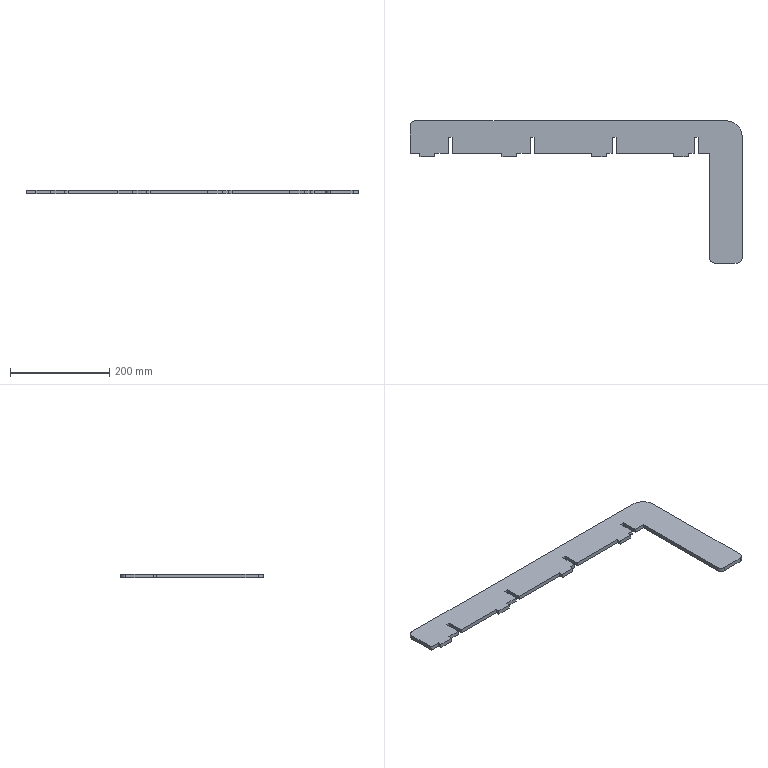Part | SolidWorks | features FlatPattern 1, SMBaseFlange 1, SheetMetal 1 | 1 solid | 44 faces | box 668 x 286 x 8 mm | volume 459100 mm3 | plane 40 | cylinder 4 | commonest cylinder face diameters 20 x3 60 x1
STEP:
#1=CARTESIAN_POINT('',(-414.372,-295.505,0.));
#2=VERTEX_POINT('',#1);
#3=CARTESIAN_POINT('',(-414.372,-350.505,0.));
#4=VERTEX_POINT('',#3);
#5=CARTESIAN_POINT('',(-414.372,-295.505,0.));
#6=DIRECTION('',(0.,-1.,0.));
#7=VECTOR('',#6,1000.);
#8=LINE('',#5,#7);
#9=EDGE_CURVE('',#2,#4,#8,.T.);
#10=ORIENTED_EDGE('',*,*,#9,.F.);
#11=CARTESIAN_POINT('',(-414.372,-295.505,-8.));
#12=VERTEX_POINT('',#11);
#13=CARTESIAN_POINT('',(-414.372,-295.505,-8.));
#14=DIRECTION('',(0.,0.,1.));
#15=VECTOR('',#14,1000.);
#16=LINE('',#13,#15);
#17=EDGE_CURVE('',#12,#2,#16,.T.);
#18=ORIENTED_EDGE('',*,*,#17,.F.);
#19=CARTESIAN_POINT('',(-414.372,-350.505,-8.));
#20=VERTEX_POINT('',#19);
#21=CARTESIAN_POINT('',(-414.372,-295.505,-8.));
#22=DIRECTION('',(0.,-1.,0.));
#23=VECTOR('',#22,1000.);
#24=LINE('',#21,#23);
#25=EDGE_CURVE('',#12,#20,#24,.T.);
#26=ORIENTED_EDGE('',*,*,#25,.T.);
#27=CARTESIAN_POINT('',(-414.372,-350.505,-8.));
#28=DIRECTION('',(0.,0.,1.));
#29=VECTOR('',#28,1000.);
#30=LINE('',#27,#29);
#31=EDGE_CURVE('',#20,#4,#30,.T.);
#32=ORIENTED_EDGE('',*,*,#31,.T.);
#33=EDGE_LOOP('',(#10,#18,#26,#32));
#34=FACE_OUTER_BOUND('',#33,.T.);
#35=CARTESIAN_POINT('',(-414.372,-295.505,-8.));
#36=DIRECTION('',(-1.,0.,0.));
#37=DIRECTION('',(0.,0.,1.));
#38=AXIS2_PLACEMENT_3D('',#35,#36,#37);
#39=PLANE('',#38);
#40=ADVANCED_FACE('',(#34),#39,.T.);
#41=CARTESIAN_POINT('',(-404.372,-285.505,0.));
#42=VERTEX_POINT('',#41);
#43=CARTESIAN_POINT('',(-404.372,-295.505,0.));
#44=DIRECTION('',(0.,0.,1.));
#45=DIRECTION('',(1.,0.,0.));
#46=AXIS2_PLACEMENT_3D('',#43,#44,#45);
#47=CIRCLE('',#46,10.);
#48=EDGE_CURVE('',#42,#2,#47,.T.);
#49=ORIENTED_EDGE('',*,*,#48,.F.);
#50=CARTESIAN_POINT('',(-404.372,-285.505,-8.));
#51=VERTEX_POINT('',#50);
#52=CARTESIAN_POINT('',(-404.372,-285.505,-8.));
#53=DIRECTION('',(0.,0.,1.));
#54=VECTOR('',#53,1000.);
#55=LINE('',#52,#54);
#56=EDGE_CURVE('',#51,#42,#55,.T.);
#57=ORIENTED_EDGE('',*,*,#56,.F.);
#58=CARTESIAN_POINT('',(-404.372,-295.505,-8.));
#59=DIRECTION('',(0.,0.,1.));
#60=DIRECTION('',(1.,0.,0.));
#61=AXIS2_PLACEMENT_3D('',#58,#59,#60);
#62=CIRCLE('',#61,10.);
#63=EDGE_CURVE('',#51,#12,#62,.T.);
#64=ORIENTED_EDGE('',*,*,#63,.T.);
#65=ORIENTED_EDGE('',*,*,#17,.T.);
#66=EDGE_LOOP('',(#49,#57,#64,#65));
#67=FACE_OUTER_BOUND('',#66,.T.);
#68=CARTESIAN_POINT('',(-404.372,-295.505,-8.));
#69=DIRECTION('',(0.,0.,1.));
#70=DIRECTION('',(1.,0.,0.));
#71=AXIS2_PLACEMENT_3D('',#68,#69,#70);
#72=CYLINDRICAL_SURFACE('',#71,10.);
#73=ADVANCED_FACE('',(#67),#72,.T.);
#74=CARTESIAN_POINT('',(223.628,-285.505,0.));
#75=VERTEX_POINT('',#74);
#76=CARTESIAN_POINT('',(223.628,-285.505,0.));
#77=DIRECTION('',(-1.,0.,0.));
#78=VECTOR('',#77,1000.);
#79=LINE('',#76,#78);
#80=EDGE_CURVE('',#75,#42,#79,.T.);
#81=ORIENTED_EDGE('',*,*,#80,.F.);
#82=CARTESIAN_POINT('',(223.628,-285.505,-8.));
#83=VERTEX_POINT('',#82);
#84=CARTESIAN_POINT('',(223.628,-285.505,-8.));
#85=DIRECTION('',(0.,0.,1.));
#86=VECTOR('',#85,1000.);
#87=LINE('',#84,#86);
#88=EDGE_CURVE('',#83,#75,#87,.T.);
#89=ORIENTED_EDGE('',*,*,#88,.F.);
#90=CARTESIAN_POINT('',(223.628,-285.505,-8.));
#91=DIRECTION('',(-1.,0.,0.));
#92=VECTOR('',#91,1000.);
#93=LINE('',#90,#92);
#94=EDGE_CURVE('',#83,#51,#93,.T.);
#95=ORIENTED_EDGE('',*,*,#94,.T.);
#96=ORIENTED_EDGE('',*,*,#56,.T.);
#97=EDGE_LOOP('',(#81,#89,#95,#96));
#98=FACE_OUTER_BOUND('',#97,.T.);
#99=CARTESIAN_POINT('',(223.628,-285.505,-8.));
#100=DIRECTION('',(0.,1.,0.));
#101=DIRECTION('',(-1.,0.,0.));
#102=AXIS2_PLACEMENT_3D('',#99,#100,#101);
#103=PLANE('',#102);
#104=ADVANCED_FACE('',(#98),#103,.T.);
#105=CARTESIAN_POINT('',(253.628,-315.505,0.));
#106=VERTEX_POINT('',#105);
#107=CARTESIAN_POINT('',(223.628,-315.505,0.));
#108=DIRECTION('',(0.,0.,1.));
#109=DIRECTION('',(1.,0.,0.));
#110=AXIS2_PLACEMENT_3D('',#107,#108,#109);
#111=CIRCLE('',#110,30.);
#112=EDGE_CURVE('',#106,#75,#111,.T.);
#113=ORIENTED_EDGE('',*,*,#112,.F.);
#114=CARTESIAN_POINT('',(253.628,-315.505,-8.));
#115=VERTEX_POINT('',#114);
#116=CARTESIAN_POINT('',(253.628,-315.505,-8.));
#117=DIRECTION('',(0.,0.,1.));
#118=VECTOR('',#117,1000.);
#119=LINE('',#116,#118);
#120=EDGE_CURVE('',#115,#106,#119,.T.);
#121=ORIENTED_EDGE('',*,*,#120,.F.);
#122=CARTESIAN_POINT('',(223.628,-315.505,-8.));
#123=DIRECTION('',(0.,0.,1.));
#124=DIRECTION('',(1.,0.,0.));
#125=AXIS2_PLACEMENT_3D('',#122,#123,#124);
#126=CIRCLE('',#125,30.);
#127=EDGE_CURVE('',#115,#83,#126,.T.);
#128=ORIENTED_EDGE('',*,*,#127,.T.);
#129=ORIENTED_EDGE('',*,*,#88,.T.);
#130=EDGE_LOOP('',(#113,#121,#128,#129));
#131=FACE_OUTER_BOUND('',#130,.T.);
#132=CARTESIAN_POINT('',(223.628,-315.505,-8.));
#133=DIRECTION('',(0.,0.,1.));
#134=DIRECTION('',(1.,0.,0.));
#135=AXIS2_PLACEMENT_3D('',#132,#133,#134);
#136=CYLINDRICAL_SURFACE('',#135,30.);
#137=ADVANCED_FACE('',(#131),#136,.T.);
#138=CARTESIAN_POINT('',(253.628,-561.505,0.));
#139=VERTEX_POINT('',#138);
#140=CARTESIAN_POINT('',(253.628,-561.505,0.));
#141=DIRECTION('',(0.,1.,0.));
#142=VECTOR('',#141,1000.);
#143=LINE('',#140,#142);
#144=EDGE_CURVE('',#139,#106,#143,.T.);
#145=ORIENTED_EDGE('',*,*,#144,.F.);
#146=CARTESIAN_POINT('',(253.628,-561.505,-8.));
#147=VERTEX_POINT('',#146);
#148=CARTESIAN_POINT('',(253.628,-561.505,-8.));
#149=DIRECTION('',(0.,0.,1.));
#150=VECTOR('',#149,1000.);
#151=LINE('',#148,#150);
#152=EDGE_CURVE('',#147,#139,#151,.T.);
#153=ORIENTED_EDGE('',*,*,#152,.F.);
#154=CARTESIAN_POINT('',(253.628,-561.505,-8.));
#155=DIRECTION('',(0.,1.,0.));
#156=VECTOR('',#155,1000.);
#157=LINE('',#154,#156);
#158=EDGE_CURVE('',#147,#115,#157,.T.);
#159=ORIENTED_EDGE('',*,*,#158,.T.);
#160=ORIENTED_EDGE('',*,*,#120,.T.);
#161=EDGE_LOOP('',(#145,#153,#159,#160));
#162=FACE_OUTER_BOUND('',#161,.T.);
#163=CARTESIAN_POINT('',(253.628,-561.505,-8.));
#164=DIRECTION('',(1.,0.,0.));
#165=DIRECTION('',(0.,0.,-1.));
#166=AXIS2_PLACEMENT_3D('',#163,#164,#165);
#167=PLANE('',#166);
#168=ADVANCED_FACE('',(#162),#167,.T.);
#169=CARTESIAN_POINT('',(243.628,-571.505,0.));
#170=VERTEX_POINT('',#169);
#171=CARTESIAN_POINT('',(243.628,-561.505,0.));
#172=DIRECTION('',(0.,0.,1.));
#173=DIRECTION('',(1.,0.,0.));
#174=AXIS2_PLACEMENT_3D('',#171,#172,#173);
#175=CIRCLE('',#174,10.);
#176=EDGE_CURVE('',#170,#139,#175,.T.);
#177=ORIENTED_EDGE('',*,*,#176,.F.);
#178=CARTESIAN_POINT('',(243.628,-571.505,-8.));
#179=VERTEX_POINT('',#178);
#180=CARTESIAN_POINT('',(243.628,-571.505,-8.));
#181=DIRECTION('',(0.,0.,1.));
#182=VECTOR('',#181,1000.);
#183=LINE('',#180,#182);
#184=EDGE_CURVE('',#179,#170,#183,.T.);
#185=ORIENTED_EDGE('',*,*,#184,.F.);
#186=CARTESIAN_POINT('',(243.628,-561.505,-8.));
#187=DIRECTION('',(0.,0.,1.));
#188=DIRECTION('',(1.,0.,0.));
#189=AXIS2_PLACEMENT_3D('',#186,#187,#188);
#190=CIRCLE('',#189,10.);
#191=EDGE_CURVE('',#179,#147,#190,.T.);
#192=ORIENTED_EDGE('',*,*,#191,.T.);
#193=ORIENTED_EDGE('',*,*,#152,.T.);
#194=EDGE_LOOP('',(#177,#185,#192,#193));
#195=FACE_OUTER_BOUND('',#194,.T.);
#196=CARTESIAN_POINT('',(243.628,-561.505,-8.));
#197=DIRECTION('',(0.,0.,1.));
#198=DIRECTION('',(1.,0.,0.));
#199=AXIS2_PLACEMENT_3D('',#196,#197,#198);
#200=CYLINDRICAL_SURFACE('',#199,10.);
#201=ADVANCED_FACE('',(#195),#200,.T.);
#202=CARTESIAN_POINT('',(198.628,-571.505,0.));
#203=VERTEX_POINT('',#202);
#204=CARTESIAN_POINT('',(198.628,-571.505,0.));
#205=DIRECTION('',(1.,0.,0.));
#206=VECTOR('',#205,1000.);
#207=LINE('',#204,#206);
#208=EDGE_CURVE('',#203,#170,#207,.T.);
#209=ORIENTED_EDGE('',*,*,#208,.F.);
#210=CARTESIAN_POINT('',(198.628,-571.505,-8.));
#211=VERTEX_POINT('',#210);
#212=CARTESIAN_POINT('',(198.628,-571.505,-8.));
#213=DIRECTION('',(0.,0.,1.));
#214=VECTOR('',#213,1000.);
#215=LINE('',#212,#214);
#216=EDGE_CURVE('',#211,#203,#215,.T.);
#217=ORIENTED_EDGE('',*,*,#216,.F.);
#218=CARTESIAN_POINT('',(198.628,-571.505,-8.));
#219=DIRECTION('',(1.,0.,0.));
#220=VECTOR('',#219,1000.);
#221=LINE('',#218,#220);
#222=EDGE_CURVE('',#211,#179,#221,.T.);
#223=ORIENTED_EDGE('',*,*,#222,.T.);
#224=ORIENTED_EDGE('',*,*,#184,.T.);
#225=EDGE_LOOP('',(#209,#217,#223,#224));
#226=FACE_OUTER_BOUND('',#225,.T.);
#227=CARTESIAN_POINT('',(198.628,-571.505,-8.));
#228=DIRECTION('',(0.,-1.,0.));
#229=DIRECTION('',(0.,0.,-1.));
#230=AXIS2_PLACEMENT_3D('',#227,#228,#229);
#231=PLANE('',#230);
#232=ADVANCED_FACE('',(#226),#231,.T.);
#233=CARTESIAN_POINT('',(188.628,-561.505,0.));
#234=VERTEX_POINT('',#233);
#235=CARTESIAN_POINT('',(198.628,-561.505,0.));
#236=DIRECTION('',(0.,0.,1.));
#237=DIRECTION('',(1.,0.,0.));
#238=AXIS2_PLACEMENT_3D('',#235,#236,#237);
#239=CIRCLE('',#238,10.);
#240=EDGE_CURVE('',#234,#203,#239,.T.);
#241=ORIENTED_EDGE('',*,*,#240,.F.);
#242=CARTESIAN_POINT('',(188.628,-561.505,-8.));
#243=VERTEX_POINT('',#242);
#244=CARTESIAN_POINT('',(188.628,-561.505,-8.));
#245=DIRECTION('',(0.,0.,1.));
#246=VECTOR('',#245,1000.);
#247=LINE('',#244,#246);
#248=EDGE_CURVE('',#243,#234,#247,.T.);
#249=ORIENTED_EDGE('',*,*,#248,.F.);
#250=CARTESIAN_POINT('',(198.628,-561.505,-8.));
#251=DIRECTION('',(0.,0.,1.));
#252=DIRECTION('',(1.,0.,0.));
#253=AXIS2_PLACEMENT_3D('',#250,#251,#252);
#254=CIRCLE('',#253,10.);
#255=EDGE_CURVE('',#243,#211,#254,.T.);
#256=ORIENTED_EDGE('',*,*,#255,.T.);
#257=ORIENTED_EDGE('',*,*,#216,.T.);
#258=EDGE_LOOP('',(#241,#249,#256,#257));
#259=FACE_OUTER_BOUND('',#258,.T.);
#260=CARTESIAN_POINT('',(198.628,-561.505,-8.));
#261=DIRECTION('',(0.,0.,1.));
#262=DIRECTION('',(1.,0.,0.));
#263=AXIS2_PLACEMENT_3D('',#260,#261,#262);
#264=CYLINDRICAL_SURFACE('',#263,10.);
#265=ADVANCED_FACE('',(#259),#264,.T.);
#266=CARTESIAN_POINT('',(188.628,-350.505,0.));
#267=VERTEX_POINT('',#266);
#268=CARTESIAN_POINT('',(188.628,-350.505,0.));
#269=DIRECTION('',(0.,-1.,0.));
#270=VECTOR('',#269,1000.);
#271=LINE('',#268,#270);
#272=EDGE_CURVE('',#267,#234,#271,.T.);
#273=ORIENTED_EDGE('',*,*,#272,.F.);
#274=CARTESIAN_POINT('',(188.628,-350.505,-8.));
#275=VERTEX_POINT('',#274);
#276=CARTESIAN_POINT('',(188.628,-350.505,-8.));
#277=DIRECTION('',(0.,0.,1.));
#278=VECTOR('',#277,1000.);
#279=LINE('',#276,#278);
#280=EDGE_CURVE('',#275,#267,#279,.T.);
#281=ORIENTED_EDGE('',*,*,#280,.F.);
#282=CARTESIAN_POINT('',(188.628,-350.505,-8.));
#283=DIRECTION('',(0.,-1.,0.));
#284=VECTOR('',#283,1000.);
#285=LINE('',#282,#284);
#286=EDGE_CURVE('',#275,#243,#285,.T.);
#287=ORIENTED_EDGE('',*,*,#286,.T.);
#288=ORIENTED_EDGE('',*,*,#248,.T.);
#289=EDGE_LOOP('',(#273,#281,#287,#288));
#290=FACE_OUTER_BOUND('',#289,.T.);
#291=CARTESIAN_POINT('',(188.628,-350.505,-8.));
#292=DIRECTION('',(-1.,0.,0.));
#293=DIRECTION('',(0.,-1.,0.));
#294=AXIS2_PLACEMENT_3D('',#291,#292,#293);
#295=PLANE('',#294);
#296=ADVANCED_FACE('',(#290),#295,.T.);
#297=CARTESIAN_POINT('',(165.628,-350.505,0.));
#298=VERTEX_POINT('',#297);
#299=CARTESIAN_POINT('',(165.628,-350.505,0.));
#300=DIRECTION('',(1.,0.,0.));
#301=VECTOR('',#300,1000.);
#302=LINE('',#299,#301);
#303=EDGE_CURVE('',#298,#267,#302,.T.);
#304=ORIENTED_EDGE('',*,*,#303,.F.);
#305=CARTESIAN_POINT('',(165.628,-350.505,-8.));
#306=VERTEX_POINT('',#305);
#307=CARTESIAN_POINT('',(165.628,-350.505,-8.));
#308=DIRECTION('',(0.,0.,1.));
#309=VECTOR('',#308,1000.);
#310=LINE('',#307,#309);
#311=EDGE_CURVE('',#306,#298,#310,.T.);
#312=ORIENTED_EDGE('',*,*,#311,.F.);
#313=CARTESIAN_POINT('',(165.628,-350.505,-8.));
#314=DIRECTION('',(1.,0.,0.));
#315=VECTOR('',#314,1000.);
#316=LINE('',#313,#315);
#317=EDGE_CURVE('',#306,#275,#316,.T.);
#318=ORIENTED_EDGE('',*,*,#317,.T.);
#319=ORIENTED_EDGE('',*,*,#280,.T.);
#320=EDGE_LOOP('',(#304,#312,#318,#319));
#321=FACE_OUTER_BOUND('',#320,.T.);
#322=CARTESIAN_POINT('',(165.628,-350.505,-8.));
#323=DIRECTION('',(0.,-1.,0.));
#324=DIRECTION('',(0.,0.,-1.));
#325=AXIS2_PLACEMENT_3D('',#322,#323,#324);
#326=PLANE('',#325);
#327=ADVANCED_FACE('',(#321),#326,.T.);
#328=CARTESIAN_POINT('',(165.628,-318.005,0.));
#329=VERTEX_POINT('',#328);
#330=CARTESIAN_POINT('',(165.628,-350.505,0.));
#331=DIRECTION('',(0.,-1.,0.));
#332=VECTOR('',#331,1000.);
#333=LINE('',#330,#332);
#334=EDGE_CURVE('',#329,#298,#333,.T.);
#335=ORIENTED_EDGE('',*,*,#334,.F.);
#336=CARTESIAN_POINT('',(165.628,-318.005,-8.));
#337=VERTEX_POINT('',#336);
#338=CARTESIAN_POINT('',(165.628,-318.005,-8.));
#339=DIRECTION('',(0.,0.,1.));
#340=VECTOR('',#339,1000.);
#341=LINE('',#338,#340);
#342=EDGE_CURVE('',#337,#329,#341,.T.);
#343=ORIENTED_EDGE('',*,*,#342,.F.);
#344=CARTESIAN_POINT('',(165.628,-350.505,-8.));
#345=DIRECTION('',(0.,-1.,0.));
#346=VECTOR('',#345,1000.);
#347=LINE('',#344,#346);
#348=EDGE_CURVE('',#337,#306,#347,.T.);
#349=ORIENTED_EDGE('',*,*,#348,.T.);
#350=ORIENTED_EDGE('',*,*,#311,.T.);
#351=EDGE_LOOP('',(#335,#343,#349,#350));
#352=FACE_OUTER_BOUND('',#351,.T.);
#353=CARTESIAN_POINT('',(165.628,-350.505,-8.));
#354=DIRECTION('',(-1.,0.,0.));
#355=DIRECTION('',(0.,-1.,0.));
#356=AXIS2_PLACEMENT_3D('',#353,#354,#355);
#357=PLANE('',#356);
#358=ADVANCED_FACE('',(#352),#357,.T.);
#359=CARTESIAN_POINT('',(157.628,-318.005,0.));
#360=VERTEX_POINT('',#359);
#361=CARTESIAN_POINT('',(165.628,-318.005,0.));
#362=DIRECTION('',(1.,0.,0.));
#363=VECTOR('',#362,1000.);
#364=LINE('',#361,#363);
#365=EDGE_CURVE('',#360,#329,#364,.T.);
#366=ORIENTED_EDGE('',*,*,#365,.F.);
#367=CARTESIAN_POINT('',(157.628,-318.005,-8.));
#368=VERTEX_POINT('',#367);
#369=CARTESIAN_POINT('',(157.628,-318.005,-8.));
#370=DIRECTION('',(0.,0.,1.));
#371=VECTOR('',#370,1000.);
#372=LINE('',#369,#371);
#373=EDGE_CURVE('',#368,#360,#372,.T.);
#374=ORIENTED_EDGE('',*,*,#373,.F.);
#375=CARTESIAN_POINT('',(165.628,-318.005,-8.));
#376=DIRECTION('',(1.,0.,0.));
#377=VECTOR('',#376,1000.);
#378=LINE('',#375,#377);
#379=EDGE_CURVE('',#368,#337,#378,.T.);
#380=ORIENTED_EDGE('',*,*,#379,.T.);
#381=ORIENTED_EDGE('',*,*,#342,.T.);
#382=EDGE_LOOP('',(#366,#374,#380,#381));
#383=FACE_OUTER_BOUND('',#382,.T.);
#384=CARTESIAN_POINT('',(165.628,-318.005,-8.));
#385=DIRECTION('',(0.,-1.,0.));
#386=DIRECTION('',(0.,0.,-1.));
#387=AXIS2_PLACEMENT_3D('',#384,#385,#386);
#388=PLANE('',#387);
#389=ADVANCED_FACE('',(#383),#388,.T.);
#390=CARTESIAN_POINT('',(157.628,-350.505,0.));
#391=VERTEX_POINT('',#390);
#392=CARTESIAN_POINT('',(157.628,-318.005,0.));
#393=DIRECTION('',(0.,1.,0.));
#394=VECTOR('',#393,1000.);
#395=LINE('',#392,#394);
#396=EDGE_CURVE('',#391,#360,#395,.T.);
#397=ORIENTED_EDGE('',*,*,#396,.F.);
#398=CARTESIAN_POINT('',(157.628,-350.505,-8.));
#399=VERTEX_POINT('',#398);
#400=CARTESIAN_POINT('',(157.628,-350.505,-8.));
#401=DIRECTION('',(0.,0.,1.));
#402=VECTOR('',#401,1000.);
#403=LINE('',#400,#402);
#404=EDGE_CURVE('',#399,#391,#403,.T.);
#405=ORIENTED_EDGE('',*,*,#404,.F.);
#406=CARTESIAN_POINT('',(157.628,-318.005,-8.));
#407=DIRECTION('',(0.,1.,0.));
#408=VECTOR('',#407,1000.);
#409=LINE('',#406,#408);
#410=EDGE_CURVE('',#399,#368,#409,.T.);
#411=ORIENTED_EDGE('',*,*,#410,.T.);
#412=ORIENTED_EDGE('',*,*,#373,.T.);
#413=EDGE_LOOP('',(#397,#405,#411,#412));
#414=FACE_OUTER_BOUND('',#413,.T.);
#415=CARTESIAN_POINT('',(157.628,-318.005,-8.));
#416=DIRECTION('',(1.,0.,0.));
#417=DIRECTION('',(0.,0.,-1.));
#418=AXIS2_PLACEMENT_3D('',#415,#416,#417);
#419=PLANE('',#418);
#420=ADVANCED_FACE('',(#414),#419,.T.);
#421=CARTESIAN_POINT('',(145.628,-350.505,0.));
#422=VERTEX_POINT('',#421);
#423=CARTESIAN_POINT('',(145.628,-350.505,0.));
#424=DIRECTION('',(1.,0.,0.));
#425=VECTOR('',#424,1000.);
#426=LINE('',#423,#425);
#427=EDGE_CURVE('',#422,#391,#426,.T.);
#428=ORIENTED_EDGE('',*,*,#427,.F.);
#429=CARTESIAN_POINT('',(145.628,-350.505,-8.));
#430=VERTEX_POINT('',#429);
#431=CARTESIAN_POINT('',(145.628,-350.505,-8.));
#432=DIRECTION('',(0.,0.,1.));
#433=VECTOR('',#432,1000.);
#434=LINE('',#431,#433);
#435=EDGE_CURVE('',#430,#422,#434,.T.);
#436=ORIENTED_EDGE('',*,*,#435,.F.);
#437=CARTESIAN_POINT('',(145.628,-350.505,-8.));
#438=DIRECTION('',(1.,0.,0.));
#439=VECTOR('',#438,1000.);
#440=LINE('',#437,#439);
#441=EDGE_CURVE('',#430,#399,#440,.T.);
#442=ORIENTED_EDGE('',*,*,#441,.T.);
#443=ORIENTED_EDGE('',*,*,#404,.T.);
#444=EDGE_LOOP('',(#428,#436,#442,#443));
#445=FACE_OUTER_BOUND('',#444,.T.);
#446=CARTESIAN_POINT('',(145.628,-350.505,-8.));
#447=DIRECTION('',(0.,-1.,0.));
#448=DIRECTION('',(0.,0.,-1.));
#449=AXIS2_PLACEMENT_3D('',#446,#447,#448);
#450=PLANE('',#449);
#451=ADVANCED_FACE('',(#445),#450,.T.);
#452=CARTESIAN_POINT('',(145.628,-358.005,0.));
#453=VERTEX_POINT('',#452);
#454=CARTESIAN_POINT('',(145.628,-350.505,0.));
#455=DIRECTION('',(0.,1.,0.));
#456=VECTOR('',#455,1000.);
#457=LINE('',#454,#456);
#458=EDGE_CURVE('',#453,#422,#457,.T.);
#459=ORIENTED_EDGE('',*,*,#458,.F.);
#460=CARTESIAN_POINT('',(145.628,-358.005,-8.));
#461=VERTEX_POINT('',#460);
#462=CARTESIAN_POINT('',(145.628,-358.005,-8.));
#463=DIRECTION('',(0.,0.,1.));
#464=VECTOR('',#463,1000.);
#465=LINE('',#462,#464);
#466=EDGE_CURVE('',#461,#453,#465,.T.);
#467=ORIENTED_EDGE('',*,*,#466,.F.);
#468=CARTESIAN_POINT('',(145.628,-350.505,-8.));
#469=DIRECTION('',(0.,1.,0.));
#470=VECTOR('',#469,1000.);
#471=LINE('',#468,#470);
#472=EDGE_CURVE('',#461,#430,#471,.T.);
#473=ORIENTED_EDGE('',*,*,#472,.T.);
#474=ORIENTED_EDGE('',*,*,#435,.T.);
#475=EDGE_LOOP('',(#459,#467,#473,#474));
#476=FACE_OUTER_BOUND('',#475,.T.);
#477=CARTESIAN_POINT('',(145.628,-350.505,-8.));
#478=DIRECTION('',(1.,0.,0.));
#479=DIRECTION('',(0.,1.,0.));
#480=AXIS2_PLACEMENT_3D('',#477,#478,#479);
#481=PLANE('',#480);
#482=ADVANCED_FACE('',(#476),#481,.T.);
#483=CARTESIAN_POINT('',(115.628,-358.005,0.));
#484=VERTEX_POINT('',#483);
#485=CARTESIAN_POINT('',(145.628,-358.005,0.));
#486=DIRECTION('',(1.,0.,0.));
#487=VECTOR('',#486,1000.);
#488=LINE('',#485,#487);
#489=EDGE_CURVE('',#484,#453,#488,.T.);
#490=ORIENTED_EDGE('',*,*,#489,.F.);
#491=CARTESIAN_POINT('',(115.628,-358.005,-8.));
#492=VERTEX_POINT('',#491);
#493=CARTESIAN_POINT('',(115.628,-358.005,-8.));
#494=DIRECTION('',(0.,0.,1.));
#495=VECTOR('',#494,1000.);
#496=LINE('',#493,#495);
#497=EDGE_CURVE('',#492,#484,#496,.T.);
#498=ORIENTED_EDGE('',*,*,#497,.F.);
#499=CARTESIAN_POINT('',(145.628,-358.005,-8.));
#500=DIRECTION('',(1.,0.,0.));
#501=VECTOR('',#500,1000.);
#502=LINE('',#499,#501);
#503=EDGE_CURVE('',#492,#461,#502,.T.);
#504=ORIENTED_EDGE('',*,*,#503,.T.);
#505=ORIENTED_EDGE('',*,*,#466,.T.);
#506=EDGE_LOOP('',(#490,#498,#504,#505));
#507=FACE_OUTER_BOUND('',#506,.T.);
#508=CARTESIAN_POINT('',(145.628,-358.005,-8.));
#509=DIRECTION('',(0.,-1.,0.));
#510=DIRECTION('',(1.,0.,0.));
#511=AXIS2_PLACEMENT_3D('',#508,#509,#510);
#512=PLANE('',#511);
#513=ADVANCED_FACE('',(#507),#512,.T.);
#514=CARTESIAN_POINT('',(115.628,-350.505,0.));
#515=VERTEX_POINT('',#514);
#516=CARTESIAN_POINT('',(115.628,-358.005,0.));
#517=DIRECTION('',(0.,-1.,0.));
#518=VECTOR('',#517,1000.);
#519=LINE('',#516,#518);
#520=EDGE_CURVE('',#515,#484,#519,.T.);
#521=ORIENTED_EDGE('',*,*,#520,.F.);
#522=CARTESIAN_POINT('',(115.628,-350.505,-8.));
#523=VERTEX_POINT('',#522);
#524=CARTESIAN_POINT('',(115.628,-350.505,-8.));
#525=DIRECTION('',(0.,0.,1.));
#526=VECTOR('',#525,1000.);
#527=LINE('',#524,#526);
#528=EDGE_CURVE('',#523,#515,#527,.T.);
#529=ORIENTED_EDGE('',*,*,#528,.F.);
#530=CARTESIAN_POINT('',(115.628,-358.005,-8.));
#531=DIRECTION('',(0.,-1.,0.));
#532=VECTOR('',#531,1000.);
#533=LINE('',#530,#532);
#534=EDGE_CURVE('',#523,#492,#533,.T.);
#535=ORIENTED_EDGE('',*,*,#534,.T.);
#536=ORIENTED_EDGE('',*,*,#497,.T.);
#537=EDGE_LOOP('',(#521,#529,#535,#536));
#538=FACE_OUTER_BOUND('',#537,.T.);
#539=CARTESIAN_POINT('',(115.628,-358.005,-8.));
#540=DIRECTION('',(-1.,0.,0.));
#541=DIRECTION('',(0.,0.,1.));
#542=AXIS2_PLACEMENT_3D('',#539,#540,#541);
#543=PLANE('',#542);
#544=ADVANCED_FACE('',(#538),#543,.T.);
#545=CARTESIAN_POINT('',(0.6284,-350.505,0.));
#546=VERTEX_POINT('',#545);
#547=CARTESIAN_POINT('',(0.6284,-350.505,0.));
#548=DIRECTION('',(1.,0.,0.));
#549=VECTOR('',#548,1000.);
#550=LINE('',#547,#549);
#551=EDGE_CURVE('',#546,#515,#550,.T.);
#552=ORIENTED_EDGE('',*,*,#551,.F.);
#553=CARTESIAN_POINT('',(0.6284,-350.505,-8.));
#554=VERTEX_POINT('',#553);
#555=CARTESIAN_POINT('',(0.6284,-350.505,-8.));
#556=DIRECTION('',(0.,0.,1.));
#557=VECTOR('',#556,1000.);
#558=LINE('',#555,#557);
#559=EDGE_CURVE('',#554,#546,#558,.T.);
#560=ORIENTED_EDGE('',*,*,#559,.F.);
#561=CARTESIAN_POINT('',(0.6284,-350.505,-8.));
#562=DIRECTION('',(1.,0.,0.));
#563=VECTOR('',#562,1000.);
#564=LINE('',#561,#563);
#565=EDGE_CURVE('',#554,#523,#564,.T.);
#566=ORIENTED_EDGE('',*,*,#565,.T.);
#567=ORIENTED_EDGE('',*,*,#528,.T.);
#568=EDGE_LOOP('',(#552,#560,#566,#567));
#569=FACE_OUTER_BOUND('',#568,.T.);
#570=CARTESIAN_POINT('',(0.6284,-350.505,-8.));
#571=DIRECTION('',(0.,-1.,0.));
#572=DIRECTION('',(0.,0.,-1.));
#573=AXIS2_PLACEMENT_3D('',#570,#571,#572);
#574=PLANE('',#573);
#575=ADVANCED_FACE('',(#569),#574,.T.);
#576=CARTESIAN_POINT('',(0.6284,-318.005,0.));
#577=VERTEX_POINT('',#576);
#578=CARTESIAN_POINT('',(0.6284,-350.505,0.));
#579=DIRECTION('',(0.,-1.,0.));
#580=VECTOR('',#579,1000.);
#581=LINE('',#578,#580);
#582=EDGE_CURVE('',#577,#546,#581,.T.);
#583=ORIENTED_EDGE('',*,*,#582,.F.);
#584=CARTESIAN_POINT('',(0.6284,-318.005,-8.));
#585=VERTEX_POINT('',#584);
#586=CARTESIAN_POINT('',(0.6284,-318.005,-8.));
#587=DIRECTION('',(0.,0.,1.));
#588=VECTOR('',#587,1000.);
#589=LINE('',#586,#588);
#590=EDGE_CURVE('',#585,#577,#589,.T.);
#591=ORIENTED_EDGE('',*,*,#590,.F.);
#592=CARTESIAN_POINT('',(0.6284,-350.505,-8.));
#593=DIRECTION('',(0.,-1.,0.));
#594=VECTOR('',#593,1000.);
#595=LINE('',#592,#594);
#596=EDGE_CURVE('',#585,#554,#595,.T.);
#597=ORIENTED_EDGE('',*,*,#596,.T.);
#598=ORIENTED_EDGE('',*,*,#559,.T.);
#599=EDGE_LOOP('',(#583,#591,#597,#598));
#600=FACE_OUTER_BOUND('',#599,.T.);
#601=CARTESIAN_POINT('',(0.6284,-350.505,-8.));
#602=DIRECTION('',(-1.,0.,0.));
#603=DIRECTION('',(0.,-1.,0.));
#604=AXIS2_PLACEMENT_3D('',#601,#602,#603);
#605=PLANE('',#604);
#606=ADVANCED_FACE('',(#600),#605,.T.);
#607=CARTESIAN_POINT('',(-7.372,-318.005,0.));
#608=VERTEX_POINT('',#607);
#609=CARTESIAN_POINT('',(0.6284,-318.005,0.));
#610=DIRECTION('',(1.,0.,0.));
#611=VECTOR('',#610,1000.);
#612=LINE('',#609,#611);
#613=EDGE_CURVE('',#608,#577,#612,.T.);
#614=ORIENTED_EDGE('',*,*,#613,.F.);
#615=CARTESIAN_POINT('',(-7.372,-318.005,-8.));
#616=VERTEX_POINT('',#615);
#617=CARTESIAN_POINT('',(-7.372,-318.005,-8.));
#618=DIRECTION('',(0.,0.,1.));
#619=VECTOR('',#618,1000.);
#620=LINE('',#617,#619);
#621=EDGE_CURVE('',#616,#608,#620,.T.);
#622=ORIENTED_EDGE('',*,*,#621,.F.);
#623=CARTESIAN_POINT('',(0.6284,-318.005,-8.));
#624=DIRECTION('',(1.,0.,0.));
#625=VECTOR('',#624,1000.);
#626=LINE('',#623,#625);
#627=EDGE_CURVE('',#616,#585,#626,.T.);
#628=ORIENTED_EDGE('',*,*,#627,.T.);
#629=ORIENTED_EDGE('',*,*,#590,.T.);
#630=EDGE_LOOP('',(#614,#622,#628,#629));
#631=FACE_OUTER_BOUND('',#630,.T.);
#632=CARTESIAN_POINT('',(0.6284,-318.005,-8.));
#633=DIRECTION('',(0.,-1.,0.));
#634=DIRECTION('',(0.,0.,-1.));
#635=AXIS2_PLACEMENT_3D('',#632,#633,#634);
#636=PLANE('',#635);
#637=ADVANCED_FACE('',(#631),#636,.T.);
#638=CARTESIAN_POINT('',(-7.372,-350.505,0.));
#639=VERTEX_POINT('',#638);
#640=CARTESIAN_POINT('',(-7.372,-318.005,0.));
#641=DIRECTION('',(0.,1.,0.));
#642=VECTOR('',#641,1000.);
#643=LINE('',#640,#642);
#644=EDGE_CURVE('',#639,#608,#643,.T.);
#645=ORIENTED_EDGE('',*,*,#644,.F.);
#646=CARTESIAN_POINT('',(-7.372,-350.505,-8.));
#647=VERTEX_POINT('',#646);
#648=CARTESIAN_POINT('',(-7.372,-350.505,-8.));
#649=DIRECTION('',(0.,0.,1.));
#650=VECTOR('',#649,1000.);
#651=LINE('',#648,#650);
#652=EDGE_CURVE('',#647,#639,#651,.T.);
#653=ORIENTED_EDGE('',*,*,#652,.F.);
#654=CARTESIAN_POINT('',(-7.372,-318.005,-8.));
#655=DIRECTION('',(0.,1.,0.));
#656=VECTOR('',#655,1000.);
#657=LINE('',#654,#656);
#658=EDGE_CURVE('',#647,#616,#657,.T.);
#659=ORIENTED_EDGE('',*,*,#658,.T.);
#660=ORIENTED_EDGE('',*,*,#621,.T.);
#661=EDGE_LOOP('',(#645,#653,#659,#660));
#662=FACE_OUTER_BOUND('',#661,.T.);
#663=CARTESIAN_POINT('',(-7.372,-318.005,-8.));
#664=DIRECTION('',(1.,0.,0.));
#665=DIRECTION('',(0.,0.,-1.));
#666=AXIS2_PLACEMENT_3D('',#663,#664,#665);
#667=PLANE('',#666);
#668=ADVANCED_FACE('',(#662),#667,.T.);
#669=CARTESIAN_POINT('',(-19.372,-350.505,0.));
#670=VERTEX_POINT('',#669);
#671=CARTESIAN_POINT('',(-19.372,-350.505,0.));
#672=DIRECTION('',(1.,0.,0.));
#673=VECTOR('',#672,1000.);
#674=LINE('',#671,#673);
#675=EDGE_CURVE('',#670,#639,#674,.T.);
#676=ORIENTED_EDGE('',*,*,#675,.F.);
#677=CARTESIAN_POINT('',(-19.372,-350.505,-8.));
#678=VERTEX_POINT('',#677);
#679=CARTESIAN_POINT('',(-19.372,-350.505,-8.));
#680=DIRECTION('',(0.,0.,1.));
#681=VECTOR('',#680,1000.);
#682=LINE('',#679,#681);
#683=EDGE_CURVE('',#678,#670,#682,.T.);
#684=ORIENTED_EDGE('',*,*,#683,.F.);
#685=CARTESIAN_POINT('',(-19.372,-350.505,-8.));
#686=DIRECTION('',(1.,0.,0.));
#687=VECTOR('',#686,1000.);
#688=LINE('',#685,#687);
#689=EDGE_CURVE('',#678,#647,#688,.T.);
#690=ORIENTED_EDGE('',*,*,#689,.T.);
#691=ORIENTED_EDGE('',*,*,#652,.T.);
#692=EDGE_LOOP('',(#676,#684,#690,#691));
#693=FACE_OUTER_BOUND('',#692,.T.);
#694=CARTESIAN_POINT('',(-19.372,-350.505,-8.));
#695=DIRECTION('',(0.,-1.,0.));
#696=DIRECTION('',(0.,0.,-1.));
#697=AXIS2_PLACEMENT_3D('',#694,#695,#696);
#698=PLANE('',#697);
#699=ADVANCED_FACE('',(#693),#698,.T.);
#700=CARTESIAN_POINT('',(-19.372,-358.005,0.));
#701=VERTEX_POINT('',#700);
#702=CARTESIAN_POINT('',(-19.372,-358.005,0.));
#703=DIRECTION('',(0.,1.,0.));
#704=VECTOR('',#703,1000.);
#705=LINE('',#702,#704);
#706=EDGE_CURVE('',#701,#670,#705,.T.);
#707=ORIENTED_EDGE('',*,*,#706,.F.);
#708=CARTESIAN_POINT('',(-19.372,-358.005,-8.));
#709=VERTEX_POINT('',#708);
#710=CARTESIAN_POINT('',(-19.372,-358.005,-8.));
#711=DIRECTION('',(0.,0.,1.));
#712=VECTOR('',#711,1000.);
#713=LINE('',#710,#712);
#714=EDGE_CURVE('',#709,#701,#713,.T.);
#715=ORIENTED_EDGE('',*,*,#714,.F.);
#716=CARTESIAN_POINT('',(-19.372,-358.005,-8.));
#717=DIRECTION('',(0.,1.,0.));
#718=VECTOR('',#717,1000.);
#719=LINE('',#716,#718);
#720=EDGE_CURVE('',#709,#678,#719,.T.);
#721=ORIENTED_EDGE('',*,*,#720,.T.);
#722=ORIENTED_EDGE('',*,*,#683,.T.);
#723=EDGE_LOOP('',(#707,#715,#721,#722));
#724=FACE_OUTER_BOUND('',#723,.T.);
#725=CARTESIAN_POINT('',(-19.372,-358.005,-8.));
#726=DIRECTION('',(1.,0.,0.));
#727=DIRECTION('',(0.,0.,-1.));
#728=AXIS2_PLACEMENT_3D('',#725,#726,#727);
#729=PLANE('',#728);
#730=ADVANCED_FACE('',(#724),#729,.T.);
#731=CARTESIAN_POINT('',(-49.372,-358.005,0.));
#732=VERTEX_POINT('',#731);
#733=CARTESIAN_POINT('',(-49.372,-358.005,0.));
#734=DIRECTION('',(1.,0.,0.));
#735=VECTOR('',#734,1000.);
#736=LINE('',#733,#735);
#737=EDGE_CURVE('',#732,#701,#736,.T.);
#738=ORIENTED_EDGE('',*,*,#737,.F.);
#739=CARTESIAN_POINT('',(-49.372,-358.005,-8.));
#740=VERTEX_POINT('',#739);
#741=CARTESIAN_POINT('',(-49.372,-358.005,-8.));
#742=DIRECTION('',(0.,0.,1.));
#743=VECTOR('',#742,1000.);
#744=LINE('',#741,#743);
#745=EDGE_CURVE('',#740,#732,#744,.T.);
#746=ORIENTED_EDGE('',*,*,#745,.F.);
#747=CARTESIAN_POINT('',(-49.372,-358.005,-8.));
#748=DIRECTION('',(1.,0.,0.));
#749=VECTOR('',#748,1000.);
#750=LINE('',#747,#749);
#751=EDGE_CURVE('',#740,#709,#750,.T.);
#752=ORIENTED_EDGE('',*,*,#751,.T.);
#753=ORIENTED_EDGE('',*,*,#714,.T.);
#754=EDGE_LOOP('',(#738,#746,#752,#753));
#755=FACE_OUTER_BOUND('',#754,.T.);
#756=CARTESIAN_POINT('',(-49.372,-358.005,-8.));
#757=DIRECTION('',(0.,-1.,0.));
#758=DIRECTION('',(1.,0.,0.));
#759=AXIS2_PLACEMENT_3D('',#756,#757,#758);
#760=PLANE('',#759);
#761=ADVANCED_FACE('',(#755),#760,.T.);
#762=CARTESIAN_POINT('',(-49.372,-350.505,0.));
#763=VERTEX_POINT('',#762);
#764=CARTESIAN_POINT('',(-49.372,-350.505,0.));
#765=DIRECTION('',(0.,-1.,0.));
#766=VECTOR('',#765,1000.);
#767=LINE('',#764,#766);
#768=EDGE_CURVE('',#763,#732,#767,.T.);
#769=ORIENTED_EDGE('',*,*,#768,.F.);
#770=CARTESIAN_POINT('',(-49.372,-350.505,-8.));
#771=VERTEX_POINT('',#770);
#772=CARTESIAN_POINT('',(-49.372,-350.505,-8.));
#773=DIRECTION('',(0.,0.,1.));
#774=VECTOR('',#773,1000.);
#775=LINE('',#772,#774);
#776=EDGE_CURVE('',#771,#763,#775,.T.);
#777=ORIENTED_EDGE('',*,*,#776,.F.);
#778=CARTESIAN_POINT('',(-49.372,-350.505,-8.));
#779=DIRECTION('',(0.,-1.,0.));
#780=VECTOR('',#779,1000.);
#781=LINE('',#778,#780);
#782=EDGE_CURVE('',#771,#740,#781,.T.);
#783=ORIENTED_EDGE('',*,*,#782,.T.);
#784=ORIENTED_EDGE('',*,*,#745,.T.);
#785=EDGE_LOOP('',(#769,#777,#783,#784));
#786=FACE_OUTER_BOUND('',#785,.T.);
#787=CARTESIAN_POINT('',(-49.372,-350.505,-8.));
#788=DIRECTION('',(-1.,0.,0.));
#789=DIRECTION('',(0.,0.,1.));
#790=AXIS2_PLACEMENT_3D('',#787,#788,#789);
#791=PLANE('',#790);
#792=ADVANCED_FACE('',(#786),#791,.T.);
#793=CARTESIAN_POINT('',(-164.372,-350.505,0.));
#794=VERTEX_POINT('',#793);
#795=CARTESIAN_POINT('',(-164.372,-350.505,0.));
#796=DIRECTION('',(1.,0.,0.));
#797=VECTOR('',#796,1000.);
#798=LINE('',#795,#797);
#799=EDGE_CURVE('',#794,#763,#798,.T.);
#800=ORIENTED_EDGE('',*,*,#799,.F.);
#801=CARTESIAN_POINT('',(-164.372,-350.505,-8.));
#802=VERTEX_POINT('',#801);
#803=CARTESIAN_POINT('',(-164.372,-350.505,-8.));
#804=DIRECTION('',(0.,0.,1.));
#805=VECTOR('',#804,1000.);
#806=LINE('',#803,#805);
#807=EDGE_CURVE('',#802,#794,#806,.T.);
#808=ORIENTED_EDGE('',*,*,#807,.F.);
#809=CARTESIAN_POINT('',(-164.372,-350.505,-8.));
#810=DIRECTION('',(1.,0.,0.));
#811=VECTOR('',#810,1000.);
#812=LINE('',#809,#811);
#813=EDGE_CURVE('',#802,#771,#812,.T.);
#814=ORIENTED_EDGE('',*,*,#813,.T.);
#815=ORIENTED_EDGE('',*,*,#776,.T.);
#816=EDGE_LOOP('',(#800,#808,#814,#815));
#817=FACE_OUTER_BOUND('',#816,.T.);
#818=CARTESIAN_POINT('',(-164.372,-350.505,-8.));
#819=DIRECTION('',(0.,-1.,0.));
#820=DIRECTION('',(0.,0.,-1.));
#821=AXIS2_PLACEMENT_3D('',#818,#819,#820);
#822=PLANE('',#821);
#823=ADVANCED_FACE('',(#817),#822,.T.);
#824=CARTESIAN_POINT('',(-164.372,-318.005,0.));
#825=VERTEX_POINT('',#824);
#826=CARTESIAN_POINT('',(-164.372,-350.505,0.));
#827=DIRECTION('',(0.,-1.,0.));
#828=VECTOR('',#827,1000.);
#829=LINE('',#826,#828);
#830=EDGE_CURVE('',#825,#794,#829,.T.);
#831=ORIENTED_EDGE('',*,*,#830,.F.);
#832=CARTESIAN_POINT('',(-164.372,-318.005,-8.));
#833=VERTEX_POINT('',#832);
#834=CARTESIAN_POINT('',(-164.372,-318.005,-8.));
#835=DIRECTION('',(0.,0.,1.));
#836=VECTOR('',#835,1000.);
#837=LINE('',#834,#836);
#838=EDGE_CURVE('',#833,#825,#837,.T.);
#839=ORIENTED_EDGE('',*,*,#838,.F.);
#840=CARTESIAN_POINT('',(-164.372,-350.505,-8.));
#841=DIRECTION('',(0.,-1.,0.));
#842=VECTOR('',#841,1000.);
#843=LINE('',#840,#842);
#844=EDGE_CURVE('',#833,#802,#843,.T.);
#845=ORIENTED_EDGE('',*,*,#844,.T.);
#846=ORIENTED_EDGE('',*,*,#807,.T.);
#847=EDGE_LOOP('',(#831,#839,#845,#846));
#848=FACE_OUTER_BOUND('',#847,.T.);
#849=CARTESIAN_POINT('',(-164.372,-350.505,-8.));
#850=DIRECTION('',(-1.,0.,0.));
#851=DIRECTION('',(0.,0.,1.));
#852=AXIS2_PLACEMENT_3D('',#849,#850,#851);
#853=PLANE('',#852);
#854=ADVANCED_FACE('',(#848),#853,.T.);
#855=CARTESIAN_POINT('',(-172.372,-318.005,0.));
#856=VERTEX_POINT('',#855);
#857=CARTESIAN_POINT('',(-164.372,-318.005,0.));
#858=DIRECTION('',(1.,0.,0.));
#859=VECTOR('',#858,1000.);
#860=LINE('',#857,#859);
#861=EDGE_CURVE('',#856,#825,#860,.T.);
#862=ORIENTED_EDGE('',*,*,#861,.F.);
#863=CARTESIAN_POINT('',(-172.372,-318.005,-8.));
#864=VERTEX_POINT('',#863);
#865=CARTESIAN_POINT('',(-172.372,-318.005,-8.));
#866=DIRECTION('',(0.,0.,1.));
#867=VECTOR('',#866,1000.);
#868=LINE('',#865,#867);
#869=EDGE_CURVE('',#864,#856,#868,.T.);
#870=ORIENTED_EDGE('',*,*,#869,.F.);
#871=CARTESIAN_POINT('',(-164.372,-318.005,-8.));
#872=DIRECTION('',(1.,0.,0.));
#873=VECTOR('',#872,1000.);
#874=LINE('',#871,#873);
#875=EDGE_CURVE('',#864,#833,#874,.T.);
#876=ORIENTED_EDGE('',*,*,#875,.T.);
#877=ORIENTED_EDGE('',*,*,#838,.T.);
#878=EDGE_LOOP('',(#862,#870,#876,#877));
#879=FACE_OUTER_BOUND('',#878,.T.);
#880=CARTESIAN_POINT('',(-164.372,-318.005,-8.));
#881=DIRECTION('',(0.,-1.,0.));
#882=DIRECTION('',(0.,0.,-1.));
#883=AXIS2_PLACEMENT_3D('',#880,#881,#882);
#884=PLANE('',#883);
#885=ADVANCED_FACE('',(#879),#884,.T.);
#886=CARTESIAN_POINT('',(-172.372,-350.505,0.));
#887=VERTEX_POINT('',#886);
#888=CARTESIAN_POINT('',(-172.372,-318.005,0.));
#889=DIRECTION('',(0.,1.,0.));
#890=VECTOR('',#889,1000.);
#891=LINE('',#888,#890);
#892=EDGE_CURVE('',#887,#856,#891,.T.);
#893=ORIENTED_EDGE('',*,*,#892,.F.);
#894=CARTESIAN_POINT('',(-172.372,-350.505,-8.));
#895=VERTEX_POINT('',#894);
#896=CARTESIAN_POINT('',(-172.372,-350.505,-8.));
#897=DIRECTION('',(0.,0.,1.));
#898=VECTOR('',#897,1000.);
#899=LINE('',#896,#898);
#900=EDGE_CURVE('',#895,#887,#899,.T.);
#901=ORIENTED_EDGE('',*,*,#900,.F.);
#902=CARTESIAN_POINT('',(-172.372,-318.005,-8.));
#903=DIRECTION('',(0.,1.,0.));
#904=VECTOR('',#903,1000.);
#905=LINE('',#902,#904);
#906=EDGE_CURVE('',#895,#864,#905,.T.);
#907=ORIENTED_EDGE('',*,*,#906,.T.);
#908=ORIENTED_EDGE('',*,*,#869,.T.);
#909=EDGE_LOOP('',(#893,#901,#907,#908));
#910=FACE_OUTER_BOUND('',#909,.T.);
#911=CARTESIAN_POINT('',(-172.372,-318.005,-8.));
#912=DIRECTION('',(1.,0.,0.));
#913=DIRECTION('',(0.,0.,-1.));
#914=AXIS2_PLACEMENT_3D('',#911,#912,#913);
#915=PLANE('',#914);
#916=ADVANCED_FACE('',(#910),#915,.T.);
#917=CARTESIAN_POINT('',(-199.372,-350.505,0.));
#918=VERTEX_POINT('',#917);
#919=CARTESIAN_POINT('',(-199.372,-350.505,0.));
#920=DIRECTION('',(1.,0.,0.));
#921=VECTOR('',#920,1000.);
#922=LINE('',#919,#921);
#923=EDGE_CURVE('',#918,#887,#922,.T.);
#924=ORIENTED_EDGE('',*,*,#923,.F.);
#925=CARTESIAN_POINT('',(-199.372,-350.505,-8.));
#926=VERTEX_POINT('',#925);
#927=CARTESIAN_POINT('',(-199.372,-350.505,-8.));
#928=DIRECTION('',(0.,0.,1.));
#929=VECTOR('',#928,1000.);
#930=LINE('',#927,#929);
#931=EDGE_CURVE('',#926,#918,#930,.T.);
#932=ORIENTED_EDGE('',*,*,#931,.F.);
#933=CARTESIAN_POINT('',(-199.372,-350.505,-8.));
#934=DIRECTION('',(1.,0.,0.));
#935=VECTOR('',#934,1000.);
#936=LINE('',#933,#935);
#937=EDGE_CURVE('',#926,#895,#936,.T.);
#938=ORIENTED_EDGE('',*,*,#937,.T.);
#939=ORIENTED_EDGE('',*,*,#900,.T.);
#940=EDGE_LOOP('',(#924,#932,#938,#939));
#941=FACE_OUTER_BOUND('',#940,.T.);
#942=CARTESIAN_POINT('',(-199.372,-350.505,-8.));
#943=DIRECTION('',(0.,-1.,0.));
#944=DIRECTION('',(0.,0.,-1.));
#945=AXIS2_PLACEMENT_3D('',#942,#943,#944);
#946=PLANE('',#945);
#947=ADVANCED_FACE('',(#941),#946,.T.);
#948=CARTESIAN_POINT('',(-199.372,-358.005,0.));
#949=VERTEX_POINT('',#948);
#950=CARTESIAN_POINT('',(-199.372,-350.505,0.));
#951=DIRECTION('',(0.,1.,0.));
#952=VECTOR('',#951,1000.);
#953=LINE('',#950,#952);
#954=EDGE_CURVE('',#949,#918,#953,.T.);
#955=ORIENTED_EDGE('',*,*,#954,.F.);
#956=CARTESIAN_POINT('',(-199.372,-358.005,-8.));
#957=VERTEX_POINT('',#956);
#958=CARTESIAN_POINT('',(-199.372,-358.005,-8.));
#959=DIRECTION('',(0.,0.,1.));
#960=VECTOR('',#959,1000.);
#961=LINE('',#958,#960);
#962=EDGE_CURVE('',#957,#949,#961,.T.);
#963=ORIENTED_EDGE('',*,*,#962,.F.);
#964=CARTESIAN_POINT('',(-199.372,-350.505,-8.));
#965=DIRECTION('',(0.,1.,0.));
#966=VECTOR('',#965,1000.);
#967=LINE('',#964,#966);
#968=EDGE_CURVE('',#957,#926,#967,.T.);
#969=ORIENTED_EDGE('',*,*,#968,.T.);
#970=ORIENTED_EDGE('',*,*,#931,.T.);
#971=EDGE_LOOP('',(#955,#963,#969,#970));
#972=FACE_OUTER_BOUND('',#971,.T.);
#973=CARTESIAN_POINT('',(-199.372,-350.505,-8.));
#974=DIRECTION('',(1.,0.,0.));
#975=DIRECTION('',(0.,0.,-1.));
#976=AXIS2_PLACEMENT_3D('',#973,#974,#975);
#977=PLANE('',#976);
#978=ADVANCED_FACE('',(#972),#977,.T.);
#979=CARTESIAN_POINT('',(-229.372,-358.005,0.));
#980=VERTEX_POINT('',#979);
#981=CARTESIAN_POINT('',(-199.372,-358.005,0.));
#982=DIRECTION('',(1.,0.,0.));
#983=VECTOR('',#982,1000.);
#984=LINE('',#981,#983);
#985=EDGE_CURVE('',#980,#949,#984,.T.);
#986=ORIENTED_EDGE('',*,*,#985,.F.);
#987=CARTESIAN_POINT('',(-229.372,-358.005,-8.));
#988=VERTEX_POINT('',#987);
#989=CARTESIAN_POINT('',(-229.372,-358.005,-8.));
#990=DIRECTION('',(0.,0.,1.));
#991=VECTOR('',#990,1000.);
#992=LINE('',#989,#991);
#993=EDGE_CURVE('',#988,#980,#992,.T.);
#994=ORIENTED_EDGE('',*,*,#993,.F.);
#995=CARTESIAN_POINT('',(-199.372,-358.005,-8.));
#996=DIRECTION('',(1.,0.,0.));
#997=VECTOR('',#996,1000.);
#998=LINE('',#995,#997);
#999=EDGE_CURVE('',#988,#957,#998,.T.);
#1000=ORIENTED_EDGE('',*,*,#999,.T.);
#1001=ORIENTED_EDGE('',*,*,#962,.T.);
#1002=EDGE_LOOP('',(#986,#994,#1000,#1001));
#1003=FACE_OUTER_BOUND('',#1002,.T.);
#1004=CARTESIAN_POINT('',(-199.372,-358.005,-8.));
#1005=DIRECTION('',(0.,-1.,0.));
#1006=DIRECTION('',(0.,0.,-1.));
#1007=AXIS2_PLACEMENT_3D('',#1004,#1005,#1006);
#1008=PLANE('',#1007);
#1009=ADVANCED_FACE('',(#1003),#1008,.T.);
#1010=CARTESIAN_POINT('',(-229.372,-350.505,0.));
#1011=VERTEX_POINT('',#1010);
#1012=CARTESIAN_POINT('',(-229.372,-358.005,0.));
#1013=DIRECTION('',(0.,-1.,0.));
#1014=VECTOR('',#1013,1000.);
#1015=LINE('',#1012,#1014);
#1016=EDGE_CURVE('',#1011,#980,#1015,.T.);
#1017=ORIENTED_EDGE('',*,*,#1016,.F.);
#1018=CARTESIAN_POINT('',(-229.372,-350.505,-8.));
#1019=VERTEX_POINT('',#1018);
#1020=CARTESIAN_POINT('',(-229.372,-350.505,-8.));
#1021=DIRECTION('',(0.,0.,1.));
#1022=VECTOR('',#1021,1000.);
#1023=LINE('',#1020,#1022);
#1024=EDGE_CURVE('',#1019,#1011,#1023,.T.);
#1025=ORIENTED_EDGE('',*,*,#1024,.F.);
#1026=CARTESIAN_POINT('',(-229.372,-358.005,-8.));
#1027=DIRECTION('',(0.,-1.,0.));
#1028=VECTOR('',#1027,1000.);
#1029=LINE('',#1026,#1028);
#1030=EDGE_CURVE('',#1019,#988,#1029,.T.);
#1031=ORIENTED_EDGE('',*,*,#1030,.T.);
#1032=ORIENTED_EDGE('',*,*,#993,.T.);
#1033=EDGE_LOOP('',(#1017,#1025,#1031,#1032));
#1034=FACE_OUTER_BOUND('',#1033,.T.);
#1035=CARTESIAN_POINT('',(-229.372,-358.005,-8.));
#1036=DIRECTION('',(-1.,0.,0.));
#1037=DIRECTION('',(0.,0.,1.));
#1038=AXIS2_PLACEMENT_3D('',#1035,#1036,#1037);
#1039=PLANE('',#1038);
#1040=ADVANCED_FACE('',(#1034),#1039,.T.);
#1041=CARTESIAN_POINT('',(-329.372,-350.505,0.));
#1042=VERTEX_POINT('',#1041);
#1043=CARTESIAN_POINT('',(-329.372,-350.505,0.));
#1044=DIRECTION('',(1.,0.,0.));
#1045=VECTOR('',#1044,1000.);
#1046=LINE('',#1043,#1045);
#1047=EDGE_CURVE('',#1042,#1011,#1046,.T.);
#1048=ORIENTED_EDGE('',*,*,#1047,.F.);
#1049=CARTESIAN_POINT('',(-329.372,-350.505,-8.));
#1050=VERTEX_POINT('',#1049);
#1051=CARTESIAN_POINT('',(-329.372,-350.505,-8.));
#1052=DIRECTION('',(0.,0.,1.));
#1053=VECTOR('',#1052,1000.);
#1054=LINE('',#1051,#1053);
#1055=EDGE_CURVE('',#1050,#1042,#1054,.T.);
#1056=ORIENTED_EDGE('',*,*,#1055,.F.);
#1057=CARTESIAN_POINT('',(-329.372,-350.505,-8.));
#1058=DIRECTION('',(1.,0.,0.));
#1059=VECTOR('',#1058,1000.);
#1060=LINE('',#1057,#1059);
#1061=EDGE_CURVE('',#1050,#1019,#1060,.T.);
#1062=ORIENTED_EDGE('',*,*,#1061,.T.);
#1063=ORIENTED_EDGE('',*,*,#1024,.T.);
#1064=EDGE_LOOP('',(#1048,#1056,#1062,#1063));
#1065=FACE_OUTER_BOUND('',#1064,.T.);
#1066=CARTESIAN_POINT('',(-329.372,-350.505,-8.));
#1067=DIRECTION('',(0.,-1.,0.));
#1068=DIRECTION('',(0.,0.,-1.));
#1069=AXIS2_PLACEMENT_3D('',#1066,#1067,#1068);
#1070=PLANE('',#1069);
#1071=ADVANCED_FACE('',(#1065),#1070,.T.);
#1072=CARTESIAN_POINT('',(-329.372,-318.005,0.));
#1073=VERTEX_POINT('',#1072);
#1074=CARTESIAN_POINT('',(-329.372,-350.505,0.));
#1075=DIRECTION('',(0.,-1.,0.));
#1076=VECTOR('',#1075,1000.);
#1077=LINE('',#1074,#1076);
#1078=EDGE_CURVE('',#1073,#1042,#1077,.T.);
#1079=ORIENTED_EDGE('',*,*,#1078,.F.);
#1080=CARTESIAN_POINT('',(-329.372,-318.005,-8.));
#1081=VERTEX_POINT('',#1080);
#1082=CARTESIAN_POINT('',(-329.372,-318.005,-8.));
#1083=DIRECTION('',(0.,0.,1.));
#1084=VECTOR('',#1083,1000.);
#1085=LINE('',#1082,#1084);
#1086=EDGE_CURVE('',#1081,#1073,#1085,.T.);
#1087=ORIENTED_EDGE('',*,*,#1086,.F.);
#1088=CARTESIAN_POINT('',(-329.372,-350.505,-8.));
#1089=DIRECTION('',(0.,-1.,0.));
#1090=VECTOR('',#1089,1000.);
#1091=LINE('',#1088,#1090);
#1092=EDGE_CURVE('',#1081,#1050,#1091,.T.);
#1093=ORIENTED_EDGE('',*,*,#1092,.T.);
#1094=ORIENTED_EDGE('',*,*,#1055,.T.);
#1095=EDGE_LOOP('',(#1079,#1087,#1093,#1094));
#1096=FACE_OUTER_BOUND('',#1095,.T.);
#1097=CARTESIAN_POINT('',(-329.372,-350.505,-8.));
#1098=DIRECTION('',(-1.,0.,0.));
#1099=DIRECTION('',(0.,0.,1.));
#1100=AXIS2_PLACEMENT_3D('',#1097,#1098,#1099);
#1101=PLANE('',#1100);
#1102=ADVANCED_FACE('',(#1096),#1101,.T.);
#1103=CARTESIAN_POINT('',(-337.372,-318.005,0.));
#1104=VERTEX_POINT('',#1103);
#1105=CARTESIAN_POINT('',(-329.372,-318.005,0.));
#1106=DIRECTION('',(1.,0.,0.));
#1107=VECTOR('',#1106,1000.);
#1108=LINE('',#1105,#1107);
#1109=EDGE_CURVE('',#1104,#1073,#1108,.T.);
#1110=ORIENTED_EDGE('',*,*,#1109,.F.);
#1111=CARTESIAN_POINT('',(-337.372,-318.005,-8.));
#1112=VERTEX_POINT('',#1111);
#1113=CARTESIAN_POINT('',(-337.372,-318.005,-8.));
#1114=DIRECTION('',(0.,0.,1.));
#1115=VECTOR('',#1114,1000.);
#1116=LINE('',#1113,#1115);
#1117=EDGE_CURVE('',#1112,#1104,#1116,.T.);
#1118=ORIENTED_EDGE('',*,*,#1117,.F.);
#1119=CARTESIAN_POINT('',(-329.372,-318.005,-8.));
#1120=DIRECTION('',(1.,0.,0.));
#1121=VECTOR('',#1120,1000.);
#1122=LINE('',#1119,#1121);
#1123=EDGE_CURVE('',#1112,#1081,#1122,.T.);
#1124=ORIENTED_EDGE('',*,*,#1123,.T.);
#1125=ORIENTED_EDGE('',*,*,#1086,.T.);
#1126=EDGE_LOOP('',(#1110,#1118,#1124,#1125));
#1127=FACE_OUTER_BOUND('',#1126,.T.);
#1128=CARTESIAN_POINT('',(-329.372,-318.005,-8.));
#1129=DIRECTION('',(0.,-1.,0.));
#1130=DIRECTION('',(0.,0.,-1.));
#1131=AXIS2_PLACEMENT_3D('',#1128,#1129,#1130);
#1132=PLANE('',#1131);
#1133=ADVANCED_FACE('',(#1127),#1132,.T.);
#1134=CARTESIAN_POINT('',(-337.372,-350.505,0.));
#1135=VERTEX_POINT('',#1134);
#1136=CARTESIAN_POINT('',(-337.372,-318.005,0.));
#1137=DIRECTION('',(0.,1.,0.));
#1138=VECTOR('',#1137,1000.);
#1139=LINE('',#1136,#1138);
#1140=EDGE_CURVE('',#1135,#1104,#1139,.T.);
#1141=ORIENTED_EDGE('',*,*,#1140,.F.);
#1142=CARTESIAN_POINT('',(-337.372,-350.505,-8.));
#1143=VERTEX_POINT('',#1142);
#1144=CARTESIAN_POINT('',(-337.372,-350.505,-8.));
#1145=DIRECTION('',(0.,0.,1.));
#1146=VECTOR('',#1145,1000.);
#1147=LINE('',#1144,#1146);
#1148=EDGE_CURVE('',#1143,#1135,#1147,.T.);
#1149=ORIENTED_EDGE('',*,*,#1148,.F.);
#1150=CARTESIAN_POINT('',(-337.372,-318.005,-8.));
#1151=DIRECTION('',(0.,1.,0.));
#1152=VECTOR('',#1151,1000.);
#1153=LINE('',#1150,#1152);
#1154=EDGE_CURVE('',#1143,#1112,#1153,.T.);
#1155=ORIENTED_EDGE('',*,*,#1154,.T.);
#1156=ORIENTED_EDGE('',*,*,#1117,.T.);
#1157=EDGE_LOOP('',(#1141,#1149,#1155,#1156));
#1158=FACE_OUTER_BOUND('',#1157,.T.);
#1159=CARTESIAN_POINT('',(-337.372,-318.005,-8.));
#1160=DIRECTION('',(1.,0.,0.));
#1161=DIRECTION('',(0.,0.,-1.));
#1162=AXIS2_PLACEMENT_3D('',#1159,#1160,#1161);
#1163=PLANE('',#1162);
#1164=ADVANCED_FACE('',(#1158),#1163,.T.);
#1165=CARTESIAN_POINT('',(-364.372,-350.505,0.));
#1166=VERTEX_POINT('',#1165);
#1167=CARTESIAN_POINT('',(-364.372,-350.505,0.));
#1168=DIRECTION('',(1.,0.,0.));
#1169=VECTOR('',#1168,1000.);
#1170=LINE('',#1167,#1169);
#1171=EDGE_CURVE('',#1166,#1135,#1170,.T.);
#1172=ORIENTED_EDGE('',*,*,#1171,.F.);
#1173=CARTESIAN_POINT('',(-364.372,-350.505,-8.));
#1174=VERTEX_POINT('',#1173);
#1175=CARTESIAN_POINT('',(-364.372,-350.505,-8.));
#1176=DIRECTION('',(0.,0.,1.));
#1177=VECTOR('',#1176,1000.);
#1178=LINE('',#1175,#1177);
#1179=EDGE_CURVE('',#1174,#1166,#1178,.T.);
#1180=ORIENTED_EDGE('',*,*,#1179,.F.);
#1181=CARTESIAN_POINT('',(-364.372,-350.505,-8.));
#1182=DIRECTION('',(1.,0.,0.));
#1183=VECTOR('',#1182,1000.);
#1184=LINE('',#1181,#1183);
#1185=EDGE_CURVE('',#1174,#1143,#1184,.T.);
#1186=ORIENTED_EDGE('',*,*,#1185,.T.);
#1187=ORIENTED_EDGE('',*,*,#1148,.T.);
#1188=EDGE_LOOP('',(#1172,#1180,#1186,#1187));
#1189=FACE_OUTER_BOUND('',#1188,.T.);
#1190=CARTESIAN_POINT('',(-364.372,-350.505,-8.));
#1191=DIRECTION('',(0.,-1.,0.));
#1192=DIRECTION('',(0.,0.,-1.));
#1193=AXIS2_PLACEMENT_3D('',#1190,#1191,#1192);
#1194=PLANE('',#1193);
#1195=ADVANCED_FACE('',(#1189),#1194,.T.);
#1196=CARTESIAN_POINT('',(-364.372,-358.005,0.));
#1197=VERTEX_POINT('',#1196);
#1198=CARTESIAN_POINT('',(-364.372,-358.005,0.));
#1199=DIRECTION('',(0.,1.,0.));
#1200=VECTOR('',#1199,1000.);
#1201=LINE('',#1198,#1200);
#1202=EDGE_CURVE('',#1197,#1166,#1201,.T.);
#1203=ORIENTED_EDGE('',*,*,#1202,.F.);
#1204=CARTESIAN_POINT('',(-364.372,-358.005,-8.));
#1205=VERTEX_POINT('',#1204);
#1206=CARTESIAN_POINT('',(-364.372,-358.005,-8.));
#1207=DIRECTION('',(0.,0.,1.));
#1208=VECTOR('',#1207,1000.);
#1209=LINE('',#1206,#1208);
#1210=EDGE_CURVE('',#1205,#1197,#1209,.T.);
#1211=ORIENTED_EDGE('',*,*,#1210,.F.);
#1212=CARTESIAN_POINT('',(-364.372,-358.005,-8.));
#1213=DIRECTION('',(0.,1.,0.));
#1214=VECTOR('',#1213,1000.);
#1215=LINE('',#1212,#1214);
#1216=EDGE_CURVE('',#1205,#1174,#1215,.T.);
#1217=ORIENTED_EDGE('',*,*,#1216,.T.);
#1218=ORIENTED_EDGE('',*,*,#1179,.T.);
#1219=EDGE_LOOP('',(#1203,#1211,#1217,#1218));
#1220=FACE_OUTER_BOUND('',#1219,.T.);
#1221=CARTESIAN_POINT('',(-364.372,-358.005,-8.));
#1222=DIRECTION('',(1.,0.,0.));
#1223=DIRECTION('',(0.,0.,-1.));
#1224=AXIS2_PLACEMENT_3D('',#1221,#1222,#1223);
#1225=PLANE('',#1224);
#1226=ADVANCED_FACE('',(#1220),#1225,.T.);
#1227=CARTESIAN_POINT('',(-394.372,-358.005,0.));
#1228=VERTEX_POINT('',#1227);
#1229=CARTESIAN_POINT('',(-394.372,-358.005,0.));
#1230=DIRECTION('',(1.,0.,0.));
#1231=VECTOR('',#1230,1000.);
#1232=LINE('',#1229,#1231);
#1233=EDGE_CURVE('',#1228,#1197,#1232,.T.);
#1234=ORIENTED_EDGE('',*,*,#1233,.F.);
#1235=CARTESIAN_POINT('',(-394.372,-358.005,-8.));
#1236=VERTEX_POINT('',#1235);
#1237=CARTESIAN_POINT('',(-394.372,-358.005,-8.));
#1238=DIRECTION('',(0.,0.,1.));
#1239=VECTOR('',#1238,1000.);
#1240=LINE('',#1237,#1239);
#1241=EDGE_CURVE('',#1236,#1228,#1240,.T.);
#1242=ORIENTED_EDGE('',*,*,#1241,.F.);
#1243=CARTESIAN_POINT('',(-394.372,-358.005,-8.));
#1244=DIRECTION('',(1.,0.,0.));
#1245=VECTOR('',#1244,1000.);
#1246=LINE('',#1243,#1245);
#1247=EDGE_CURVE('',#1236,#1205,#1246,.T.);
#1248=ORIENTED_EDGE('',*,*,#1247,.T.);
#1249=ORIENTED_EDGE('',*,*,#1210,.T.);
#1250=EDGE_LOOP('',(#1234,#1242,#1248,#1249));
#1251=FACE_OUTER_BOUND('',#1250,.T.);
#1252=CARTESIAN_POINT('',(-394.372,-358.005,-8.));
#1253=DIRECTION('',(0.,-1.,0.));
#1254=DIRECTION('',(0.,0.,-1.));
#1255=AXIS2_PLACEMENT_3D('',#1252,#1253,#1254);
#1256=PLANE('',#1255);
#1257=ADVANCED_FACE('',(#1251),#1256,.T.);
#1258=CARTESIAN_POINT('',(-394.372,-350.505,0.));
#1259=VERTEX_POINT('',#1258);
#1260=CARTESIAN_POINT('',(-394.372,-350.505,0.));
#1261=DIRECTION('',(0.,-1.,0.));
#1262=VECTOR('',#1261,1000.);
#1263=LINE('',#1260,#1262);
#1264=EDGE_CURVE('',#1259,#1228,#1263,.T.);
#1265=ORIENTED_EDGE('',*,*,#1264,.F.);
#1266=CARTESIAN_POINT('',(-394.372,-350.505,-8.));
#1267=VERTEX_POINT('',#1266);
#1268=CARTESIAN_POINT('',(-394.372,-350.505,-8.));
#1269=DIRECTION('',(0.,0.,1.));
#1270=VECTOR('',#1269,1000.);
#1271=LINE('',#1268,#1270);
#1272=EDGE_CURVE('',#1267,#1259,#1271,.T.);
#1273=ORIENTED_EDGE('',*,*,#1272,.F.);
#1274=CARTESIAN_POINT('',(-394.372,-350.505,-8.));
#1275=DIRECTION('',(0.,-1.,0.));
#1276=VECTOR('',#1275,1000.);
#1277=LINE('',#1274,#1276);
#1278=EDGE_CURVE('',#1267,#1236,#1277,.T.);
#1279=ORIENTED_EDGE('',*,*,#1278,.T.);
#1280=ORIENTED_EDGE('',*,*,#1241,.T.);
#1281=EDGE_LOOP('',(#1265,#1273,#1279,#1280));
#1282=FACE_OUTER_BOUND('',#1281,.T.);
#1283=CARTESIAN_POINT('',(-394.372,-350.505,-8.));
#1284=DIRECTION('',(-1.,0.,0.));
#1285=DIRECTION('',(0.,0.,1.));
#1286=AXIS2_PLACEMENT_3D('',#1283,#1284,#1285);
#1287=PLANE('',#1286);
#1288=ADVANCED_FACE('',(#1282),#1287,.T.);
#1289=CARTESIAN_POINT('',(-414.372,-350.505,0.));
#1290=DIRECTION('',(1.,0.,0.));
#1291=VECTOR('',#1290,1000.);
#1292=LINE('',#1289,#1291);
#1293=EDGE_CURVE('',#4,#1259,#1292,.T.);
#1294=ORIENTED_EDGE('',*,*,#1293,.F.);
#1295=ORIENTED_EDGE('',*,*,#31,.F.);
#1296=CARTESIAN_POINT('',(-414.372,-350.505,-8.));
#1297=DIRECTION('',(1.,0.,0.));
#1298=VECTOR('',#1297,1000.);
#1299=LINE('',#1296,#1298);
#1300=EDGE_CURVE('',#20,#1267,#1299,.T.);
#1301=ORIENTED_EDGE('',*,*,#1300,.T.);
#1302=ORIENTED_EDGE('',*,*,#1272,.T.);
#1303=EDGE_LOOP('',(#1294,#1295,#1301,#1302));
#1304=FACE_OUTER_BOUND('',#1303,.T.);
#1305=CARTESIAN_POINT('',(-414.372,-350.505,-8.));
#1306=DIRECTION('',(0.,-1.,0.));
#1307=DIRECTION('',(0.,0.,-1.));
#1308=AXIS2_PLACEMENT_3D('',#1305,#1306,#1307);
#1309=PLANE('',#1308);
#1310=ADVANCED_FACE('',(#1304),#1309,.T.);
#1311=ORIENTED_EDGE('',*,*,#25,.F.);
#1312=ORIENTED_EDGE('',*,*,#63,.F.);
#1313=ORIENTED_EDGE('',*,*,#94,.F.);
#1314=ORIENTED_EDGE('',*,*,#127,.F.);
#1315=ORIENTED_EDGE('',*,*,#158,.F.);
#1316=ORIENTED_EDGE('',*,*,#191,.F.);
#1317=ORIENTED_EDGE('',*,*,#222,.F.);
#1318=ORIENTED_EDGE('',*,*,#255,.F.);
#1319=ORIENTED_EDGE('',*,*,#286,.F.);
#1320=ORIENTED_EDGE('',*,*,#317,.F.);
#1321=ORIENTED_EDGE('',*,*,#348,.F.);
#1322=ORIENTED_EDGE('',*,*,#379,.F.);
#1323=ORIENTED_EDGE('',*,*,#410,.F.);
#1324=ORIENTED_EDGE('',*,*,#441,.F.);
#1325=ORIENTED_EDGE('',*,*,#472,.F.);
#1326=ORIENTED_EDGE('',*,*,#503,.F.);
#1327=ORIENTED_EDGE('',*,*,#534,.F.);
#1328=ORIENTED_EDGE('',*,*,#565,.F.);
#1329=ORIENTED_EDGE('',*,*,#596,.F.);
#1330=ORIENTED_EDGE('',*,*,#627,.F.);
#1331=ORIENTED_EDGE('',*,*,#658,.F.);
#1332=ORIENTED_EDGE('',*,*,#689,.F.);
#1333=ORIENTED_EDGE('',*,*,#720,.F.);
#1334=ORIENTED_EDGE('',*,*,#751,.F.);
#1335=ORIENTED_EDGE('',*,*,#782,.F.);
#1336=ORIENTED_EDGE('',*,*,#813,.F.);
#1337=ORIENTED_EDGE('',*,*,#844,.F.);
#1338=ORIENTED_EDGE('',*,*,#875,.F.);
#1339=ORIENTED_EDGE('',*,*,#906,.F.);
#1340=ORIENTED_EDGE('',*,*,#937,.F.);
#1341=ORIENTED_EDGE('',*,*,#968,.F.);
#1342=ORIENTED_EDGE('',*,*,#999,.F.);
#1343=ORIENTED_EDGE('',*,*,#1030,.F.);
#1344=ORIENTED_EDGE('',*,*,#1061,.F.);
#1345=ORIENTED_EDGE('',*,*,#1092,.F.);
#1346=ORIENTED_EDGE('',*,*,#1123,.F.);
#1347=ORIENTED_EDGE('',*,*,#1154,.F.);
#1348=ORIENTED_EDGE('',*,*,#1185,.F.);
#1349=ORIENTED_EDGE('',*,*,#1216,.F.);
#1350=ORIENTED_EDGE('',*,*,#1247,.F.);
#1351=ORIENTED_EDGE('',*,*,#1278,.F.);
#1352=ORIENTED_EDGE('',*,*,#1300,.F.);
#1353=EDGE_LOOP('',(#1311,#1312,#1313,#1314,#1315,#1316,#1317,#1318,#1319,#1320,#1321,#1322,#1323,#1324,#1325,#1326,#1327,#1328,#1329,#1330,#1331,#1332,#1333,#1334,#1335,#1336,#1337,#1338,#1339,#1340,#1341,#1342,#1343,#1344,#1345,#1346,#1347,#1348,#1349,#1350,#1351,#1352));
#1354=FACE_OUTER_BOUND('',#1353,.T.);
#1355=CARTESIAN_POINT('',(198.628,-561.505,-8.));
#1356=DIRECTION('',(0.,0.,1.));
#1357=DIRECTION('',(1.,0.,0.));
#1358=AXIS2_PLACEMENT_3D('',#1355,#1356,#1357);
#1359=PLANE('',#1358);
#1360=ADVANCED_FACE('',(#1354),#1359,.F.);
#1361=ORIENTED_EDGE('',*,*,#9,.T.);
#1362=ORIENTED_EDGE('',*,*,#1293,.T.);
#1363=ORIENTED_EDGE('',*,*,#1264,.T.);
#1364=ORIENTED_EDGE('',*,*,#1233,.T.);
#1365=ORIENTED_EDGE('',*,*,#1202,.T.);
#1366=ORIENTED_EDGE('',*,*,#1171,.T.);
#1367=ORIENTED_EDGE('',*,*,#1140,.T.);
#1368=ORIENTED_EDGE('',*,*,#1109,.T.);
#1369=ORIENTED_EDGE('',*,*,#1078,.T.);
#1370=ORIENTED_EDGE('',*,*,#1047,.T.);
#1371=ORIENTED_EDGE('',*,*,#1016,.T.);
#1372=ORIENTED_EDGE('',*,*,#985,.T.);
#1373=ORIENTED_EDGE('',*,*,#954,.T.);
#1374=ORIENTED_EDGE('',*,*,#923,.T.);
#1375=ORIENTED_EDGE('',*,*,#892,.T.);
#1376=ORIENTED_EDGE('',*,*,#861,.T.);
#1377=ORIENTED_EDGE('',*,*,#830,.T.);
#1378=ORIENTED_EDGE('',*,*,#799,.T.);
#1379=ORIENTED_EDGE('',*,*,#768,.T.);
#1380=ORIENTED_EDGE('',*,*,#737,.T.);
#1381=ORIENTED_EDGE('',*,*,#706,.T.);
#1382=ORIENTED_EDGE('',*,*,#675,.T.);
#1383=ORIENTED_EDGE('',*,*,#644,.T.);
#1384=ORIENTED_EDGE('',*,*,#613,.T.);
#1385=ORIENTED_EDGE('',*,*,#582,.T.);
#1386=ORIENTED_EDGE('',*,*,#551,.T.);
#1387=ORIENTED_EDGE('',*,*,#520,.T.);
#1388=ORIENTED_EDGE('',*,*,#489,.T.);
#1389=ORIENTED_EDGE('',*,*,#458,.T.);
#1390=ORIENTED_EDGE('',*,*,#427,.T.);
#1391=ORIENTED_EDGE('',*,*,#396,.T.);
#1392=ORIENTED_EDGE('',*,*,#365,.T.);
#1393=ORIENTED_EDGE('',*,*,#334,.T.);
#1394=ORIENTED_EDGE('',*,*,#303,.T.);
#1395=ORIENTED_EDGE('',*,*,#272,.T.);
#1396=ORIENTED_EDGE('',*,*,#240,.T.);
#1397=ORIENTED_EDGE('',*,*,#208,.T.);
#1398=ORIENTED_EDGE('',*,*,#176,.T.);
#1399=ORIENTED_EDGE('',*,*,#144,.T.);
#1400=ORIENTED_EDGE('',*,*,#112,.T.);
#1401=ORIENTED_EDGE('',*,*,#80,.T.);
#1402=ORIENTED_EDGE('',*,*,#48,.T.);
#1403=EDGE_LOOP('',(#1361,#1362,#1363,#1364,#1365,#1366,#1367,#1368,#1369,#1370,#1371,#1372,#1373,#1374,#1375,#1376,#1377,#1378,#1379,#1380,#1381,#1382,#1383,#1384,#1385,#1386,#1387,#1388,#1389,#1390,#1391,#1392,#1393,#1394,#1395,#1396,#1397,#1398,#1399,#1400,#1401,#1402));
#1404=FACE_OUTER_BOUND('',#1403,.T.);
#1405=CARTESIAN_POINT('',(198.628,-561.505,0.));
#1406=DIRECTION('',(0.,0.,1.));
#1407=DIRECTION('',(1.,0.,0.));
#1408=AXIS2_PLACEMENT_3D('',#1405,#1406,#1407);
#1409=PLANE('',#1408);
#1410=ADVANCED_FACE('',(#1404),#1409,.T.);
#1411=CLOSED_SHELL('',(#40,#73,#104,#137,#168,#201,#232,#265,#296,#327,#358,#389,#420,#451,#482,#513,#544,#575,#606,#637,#668,#699,#730,#761,#792,#823,#854,#885,#916,#947,#978,#1009,#1040,#1071,#1102,#1133,#1164,#1195,#1226,#1257,#1288,#1310,#1360,#1410));
#1412=MANIFOLD_SOLID_BREP('',#1411);
#1413=CARTESIAN_POINT('',(0.,0.,0.));
#1414=DIRECTION('',(0.,0.,1.));
#1415=DIRECTION('',(1.,0.,0.));
#1416=AXIS2_PLACEMENT_3D('',#1413,#1414,#1415);
#1417=(LENGTH_UNIT()NAMED_UNIT(*)SI_UNIT(.MILLI.,.METRE.));
#1418=UNCERTAINTY_MEASURE_WITH_UNIT(LENGTH_MEASURE(0.00001),#1417,'','');
#1419=(NAMED_UNIT(*)PLANE_ANGLE_UNIT()SI_UNIT($,.RADIAN.));
#1420=(NAMED_UNIT(*)SI_UNIT($,.STERADIAN.)SOLID_ANGLE_UNIT());
#1421=(GEOMETRIC_REPRESENTATION_CONTEXT(3)GLOBAL_UNCERTAINTY_ASSIGNED_CONTEXT((#1418))GLOBAL_UNIT_ASSIGNED_CONTEXT((#1417,#1419,#1420))REPRESENTATION_CONTEXT('',''));
#1422=ADVANCED_BREP_SHAPE_REPRESENTATION('',(#1412,#1416),#1421);